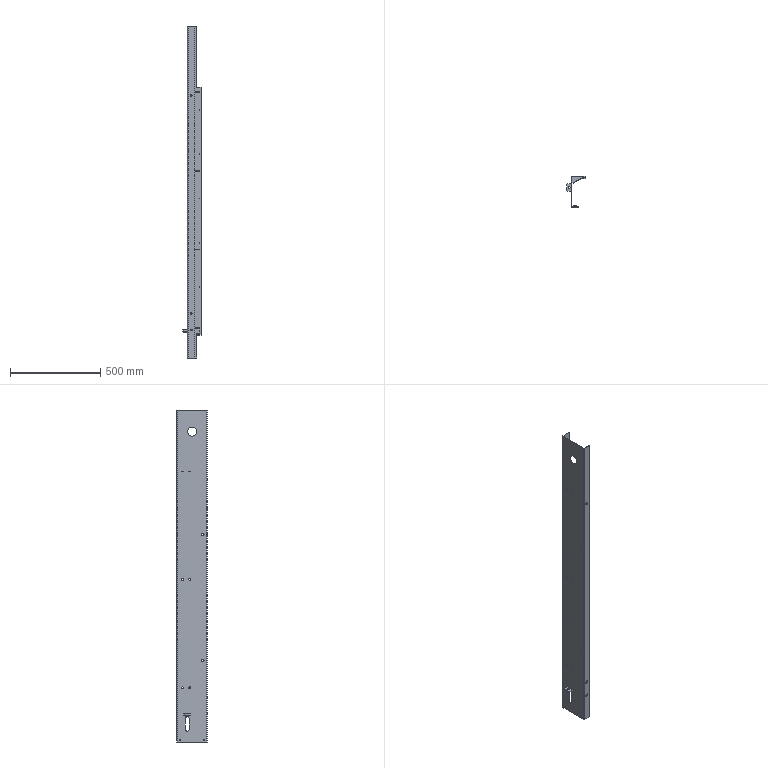Part | SolidWorks | features Cut 1, ICE 1, MirrorStock 1 | 10 solids | 200 faces | box 100 x 170 x 1838 mm | volume 1266311 mm3 | plane 88 | cone 56 | cylinder 56 | commonest cylinder face diameters 10.5 x18 4.5 x12 10 x8 6 x4 13 x4 20 x3